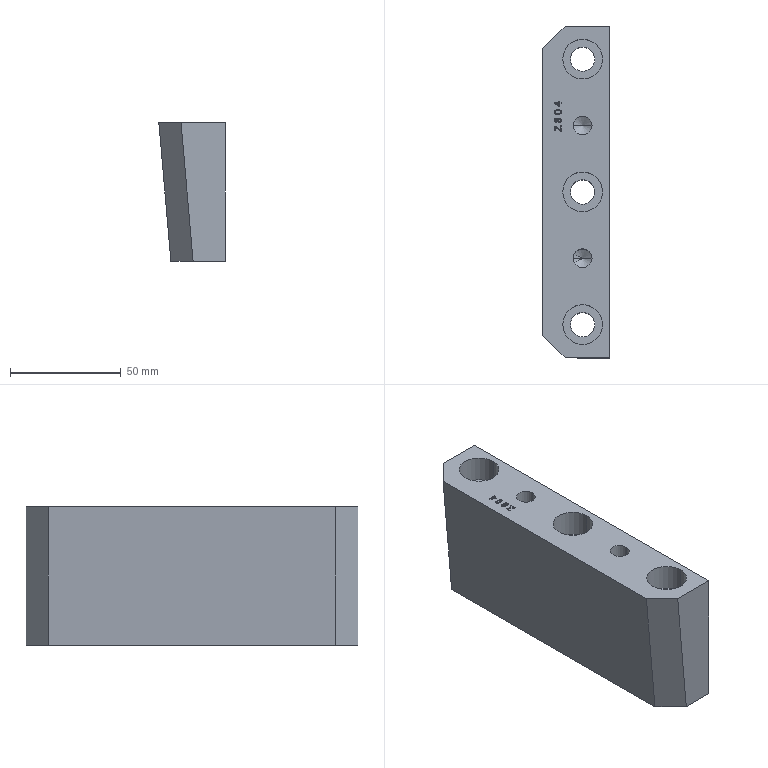Part | Creo | 1 solid | 118 faces | box 30 x 150 x 62.5 mm | volume 222678 mm3 | other 57 | plane 39 | cylinder 18 | cone 4 | commonest cylinder face diameters 11 x6 18 x6 8.5 x4 1.666 x1 45.582 x1